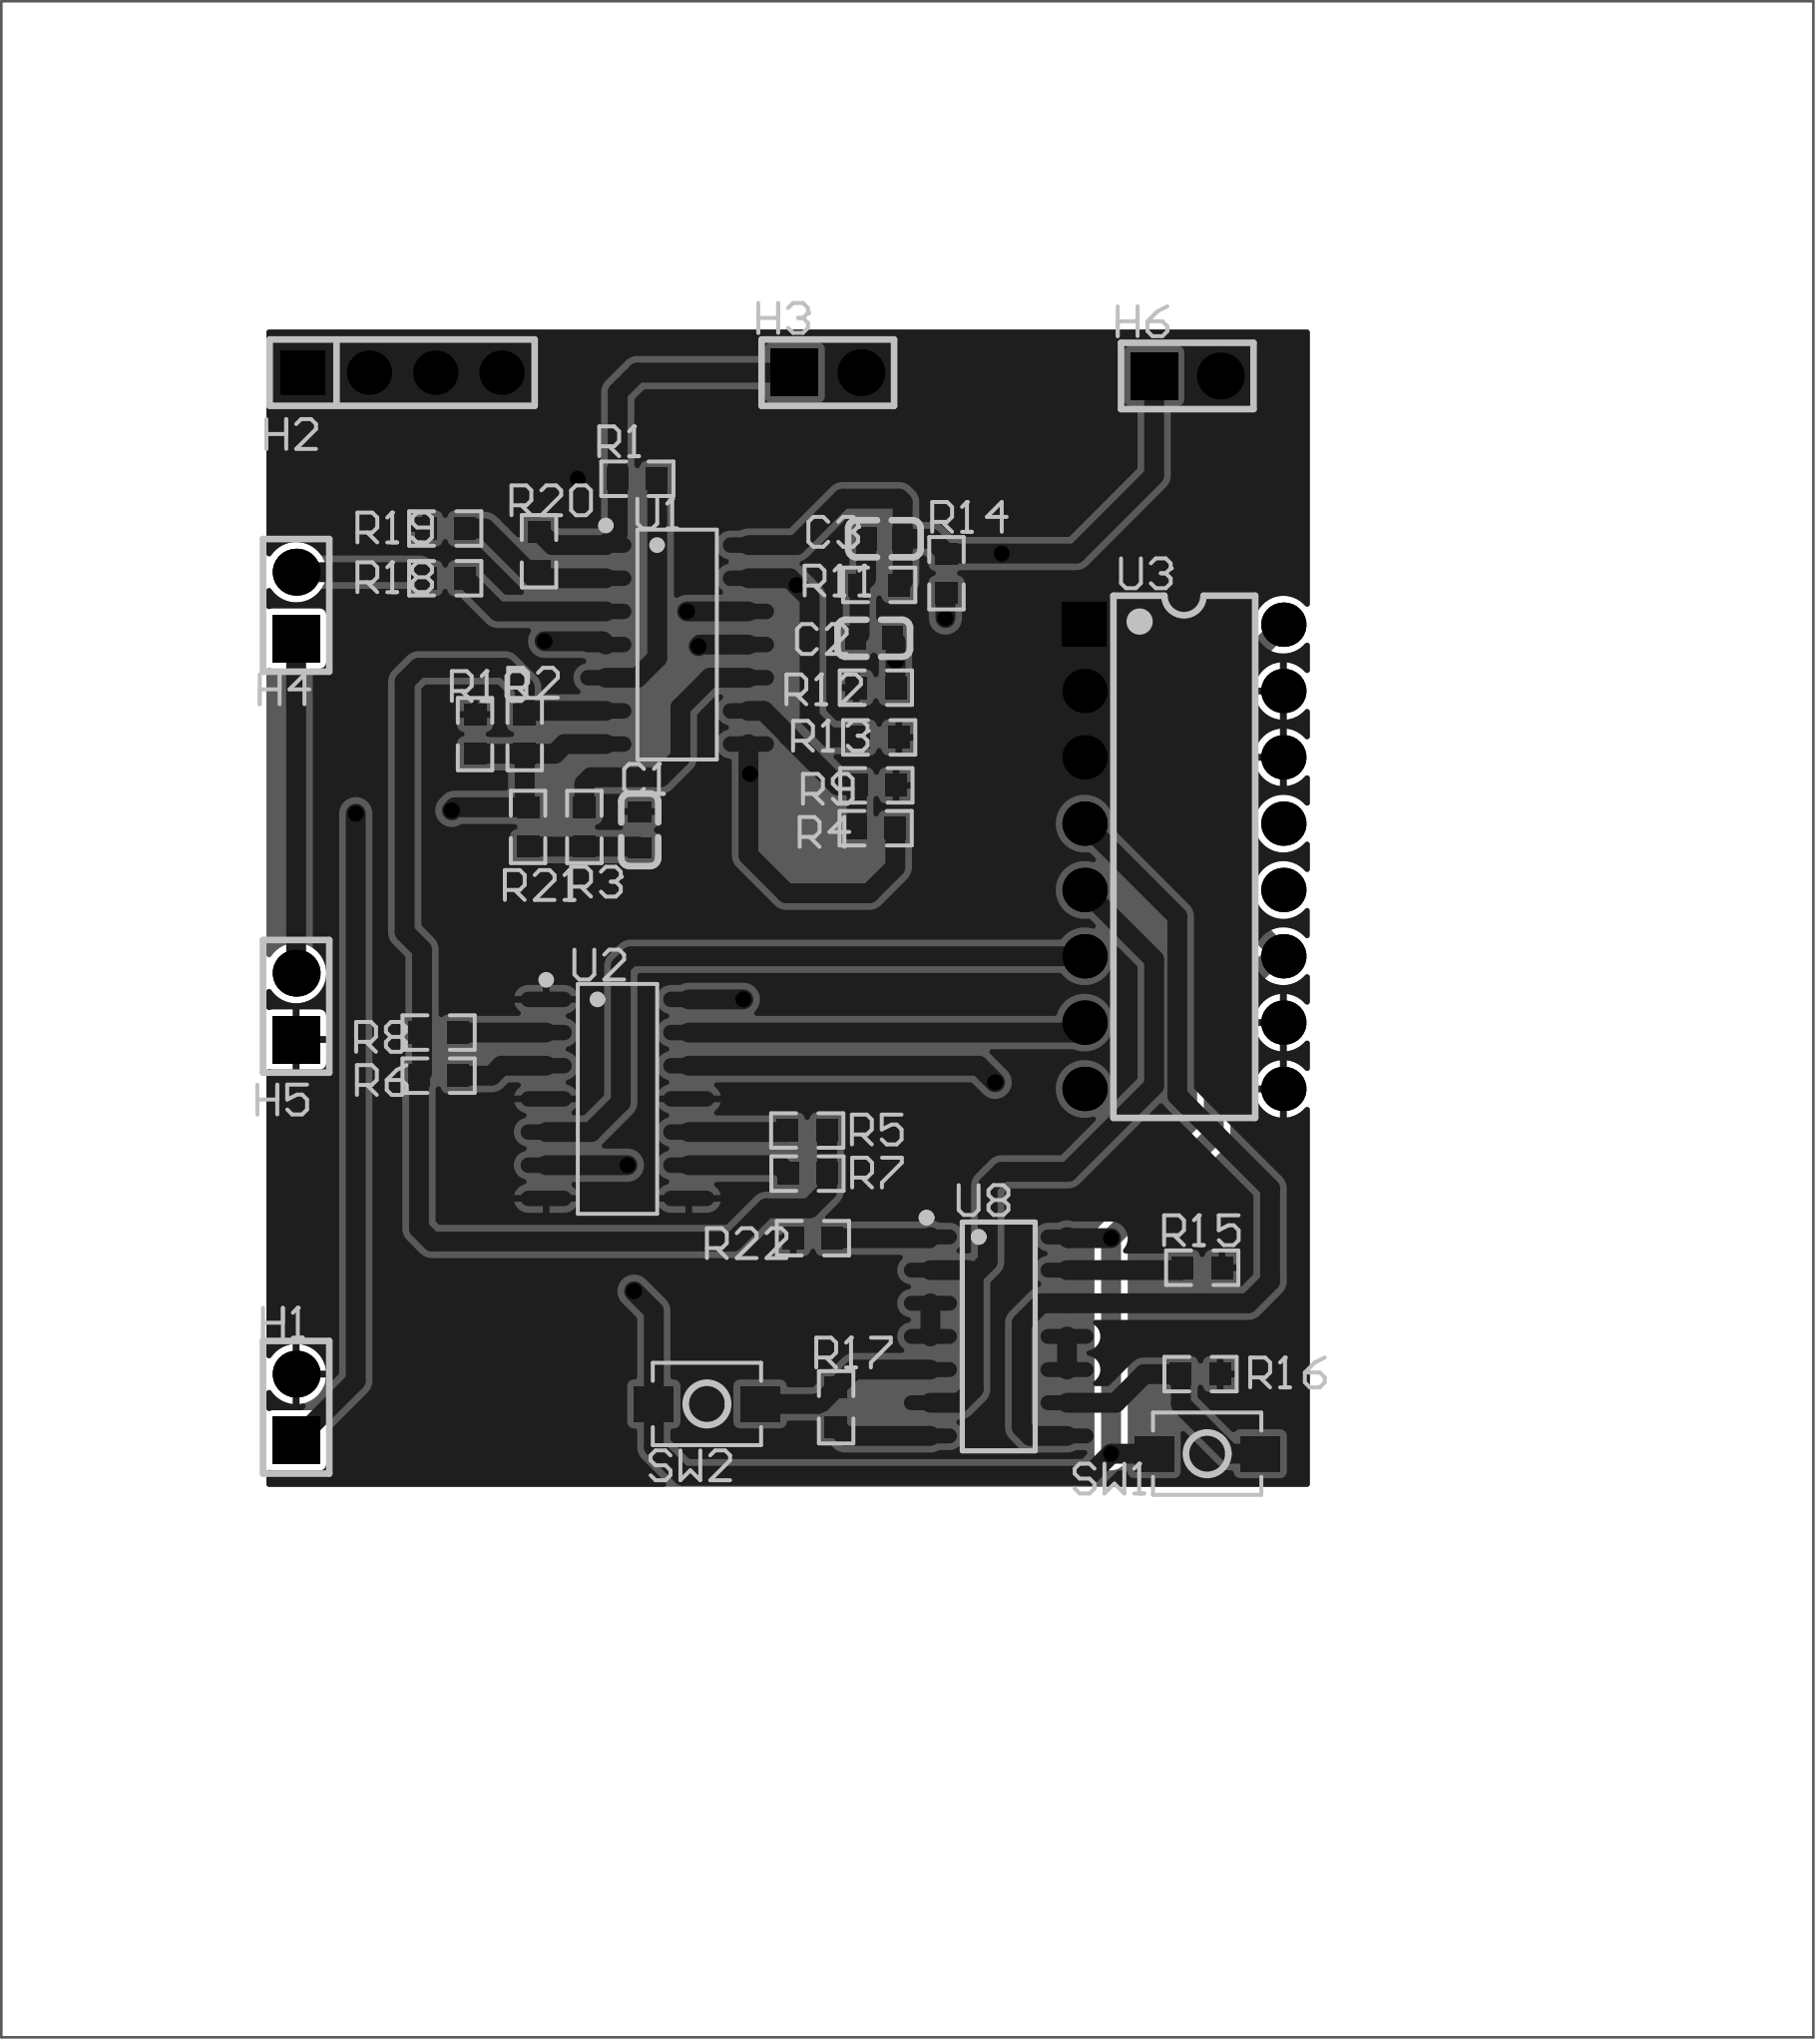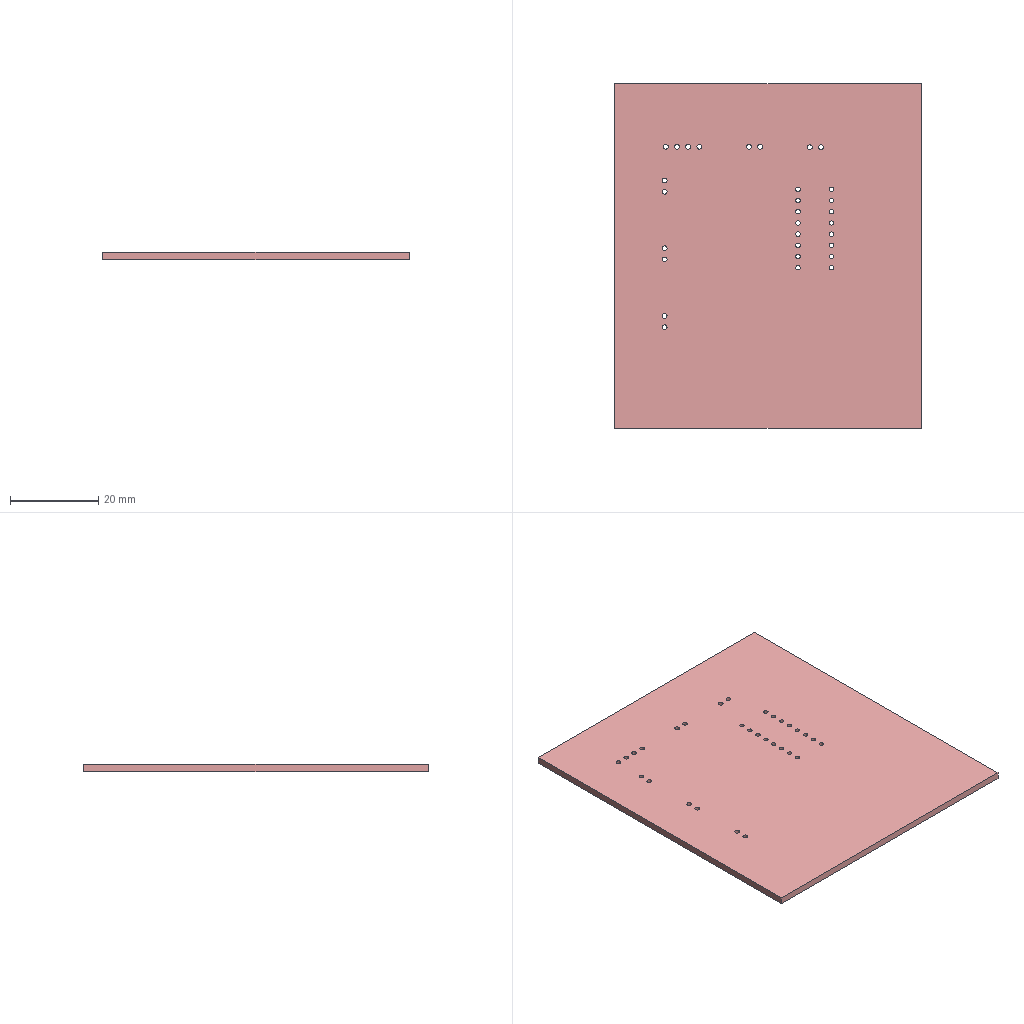Circuit board layout | Altium Designer | box 69.5 x 78 x 1.6 mm
Layer stack:
# Altium Designer layer stack of  (unit mm; dielectric type: 0 none, 1 core, 2 prepreg, 3 surface material)
index,name,kind,layer,copper_thickness_mm,dielectric_type,dielectric_thickness_mm,dielectric_material,dielectric_constant
0,Top Paste Mask Layer,other,,,,,,
1,Top Silkscreen Layer,other,,,,,,
2,Top Solder Mask Layer,dielectric,,,3,0.01,,3.3
3,Top Layer,copper,Top Layer,0.035,,,,
4,Dielectric1,dielectric,,,3,1.51,FR4,4.5
5,Bottom Layer,copper,Bottom Layer,0.035,,,,
6,Bottom Solder Mask Layer,dielectric,,,3,0.01,,3.3
7,Bottom Silkscreen Layer,other,,,,,,
8,Bottom Paste Mask Layer,other,,,,,,
# drill layer pairs: low layer,high layer
drill_pair,Top Layer,Bottom Layer
Part placement:
Designator,Comment,Layer,Footprint,Center-X(mm),Center-Y(mm),Rotation
C1,10nF,TopLayer,C0603,94.323,116.095,270
C2,100nF,TopLayer,C0603,103.298,123.433,180
C3,100nF,TopLayer,C0603,103.704,127.243,0
H1,,TopLayer,HDR-TH_2P-P2.54-V-M-1,81.153,93.98,90
H2,,TopLayer,HDR-TH_4P-P2.54-V-M,85.217,133.604,0
H3,,TopLayer,HDR-TH_2P-P2.54-V-M-1,101.537,133.604,0
H4,,TopLayer,HDR-TH_2P-P2.54-V-M-1,81.153,124.692,90
H5,,TopLayer,HDR-TH_2P-P2.54-V-M-1,81.153,109.336,90
H6,,TopLayer,HDR-TH_2P-P2.54-V-M-1,115.316,133.477,0
R1,15K,TopLayer,R0603,94.234,129.54,0
R2,1200K,TopLayer,R0603,89.916,119.761,270
R3,47K,TopLayer,R0603,92.202,116.205,90
R4,120K,TopLayer,R0603,103.37,116.157,0
R5,80K,TopLayer,R0603,100.746,104.58,0
R6,40K,TopLayer,R0603,86.614,106.68,180
R7,20K,TopLayer,R0603,100.755,102.929,0
R8,10K,TopLayer,R0603,86.614,108.331,180
R9,230K,TopLayer,R0603,103.398,117.798,180
R10,80K,TopLayer,R0603,88.011,119.761,270
R11,15K,TopLayer,R0603,103.505,125.476,0
R12,15K,TopLayer,R0603,103.378,121.539,0
R13,80K,TopLayer,R0603,103.505,119.634,180
R14,51K,TopLayer,R0603,106.084,125.922,270
R15,15K,TopLayer,R0603,115.889,99.326,0
R16,15K,TopLayer,R0603,115.824,95.25,180
R17,1K,TopLayer,R0603,101.854,93.98,90
R18,10K,TopLayer,R0603,86.868,125.73,0
R19,10K,TopLayer,R0603,86.868,127.635,0
R20,90K,TopLayer,R0603,90.463,126.765,90
R21,120K,TopLayer,R0603,90.043,116.205,270
R22,15K,TopLayer,R0603,100.965,100.457,180
SW1,,TopLayer,Key_SMD_3x4x2,116.078,92.202,180
SW2,,TopLayer,Key_SMD_3x4x2,96.901,94.107,180
U2,CD4066BD,TopLayer,SOP-14_L8.6-W3.9-P1.27-LS6.0-BL,93.472,105.791,270
U3,NTE74193,TopLayer,PDIP-16_L19.7-W6.6-P2.54-LS7.6-BL,115.189,115.062,270
U1,LM324ADR,TopLayer,SOP-14_L8.6-W3.9-P1.27-LS6.0-BL,95.758,123.19,270
U8,SN74LS00DR,TopLayer,SOIC-14_L8.7-W3.9-P1.27-LS6.0-BL,108.088,96.693,270
Pad and via stacks:
# Altium Designer via and pad stacks of  (unit mm). Each distinct definition once, with the count of objects using it.
# via: kind,start_layer,end_layer,hole_mm,diameter_mm,mode(0 simple;1 top-mid-bottom;2 full stack),diameter_per_layer,count,example_net
# pad: kind,layer,hole_mm,hole_type(0 round;1 square;2 slot),plating,top_size,top_shape(1 round;2 rect;3 octagon;9 rounded rect),mid_size,bottom_size,mode,footprint,size_per_layer,count,example
pad,Top Layer,0,0,plated,0.8x0.9,2,0.8x0.9,0.8x0.9,0,C0603,,6,C1.2
pad,Top Layer,0,0,plated,0.8065x0.864,2,0.8065x0.864,0.8065x0.864,0,R0603,,44,R1.2
pad,Top Layer,0,0,plated,1.53x1.36,2,1.53x1.36,1.53x1.36,0,Key_SMD_3x4x2,,4,SW1.1
pad,Top Layer,0,0,plated,0.595x1.968,1,0.595x1.968,0.595x1.968,0,SOP-14_L8.6-W3.9-P1.27-LS6.0-BL,,28,U2.1
pad,Top Layer,0,0,plated,0.574x2.038,1,0.574x2.038,0.574x2.038,0,SOIC-14_L8.7-W3.9-P1.27-LS6.0-BL,,14,U8.8
pad,Multi-Layer,1.1,0,plated,1.8x1.8,1,1.8x1.8,1.8x1.8,0,HDR-TH_2P-P2.54-V-M-1,,5,H1.2
pad,Multi-Layer,1.1,0,plated,1.8x1.8,2,1.8x1.8,1.8x1.8,0,HDR-TH_2P-P2.54-V-M-1,,5,H1.1
pad,Multi-Layer,1.1,0,plated,1.7x1.7,2,1.7x1.7,1.7x1.7,0,HDR-TH_4P-P2.54-V-M,,1,H2.1
pad,Multi-Layer,1.1,0,plated,1.7x1.7,1,1.7x1.7,1.7x1.7,0,HDR-TH_4P-P2.54-V-M,,3,H2.2
pad,Multi-Layer,1,0,plated,1.7x1.7,2,1.7x1.7,1.7x1.7,0,PDIP-16_L19.7-W6.6-P2.54-LS7.6-BL,,1,U3.1
pad,Multi-Layer,1,0,plated,1.7x1.7,1,1.7x1.7,1.7x1.7,0,PDIP-16_L19.7-W6.6-P2.54-LS7.6-BL,,15,U3.2
via,Top Layer,Bottom Layer,0.3048,0.61,0,,17,5V
Copper pours:
name,layer,net,type(0 solid;1 hatched;2 none)
Top Layer-GND,Top Layer,GND,0
Bottom Layer-GND,Bottom Layer,GND,0